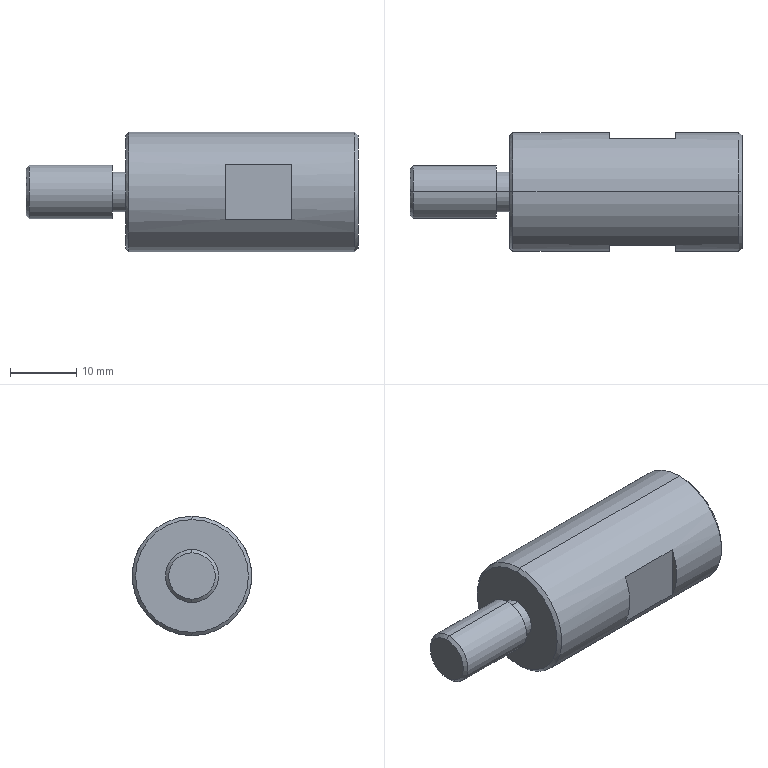Part | STEP file | PN_0032 Shaft_Default | 1 solid | 26 faces | box 50 x 18 x 18 mm | volume 8746 mm3 | plane 10 | cylinder 8 | cone 8 | commonest cylinder face diameters 6 x2 6.8 x2 8 x2 18 x2
STEP:
#1=CARTESIAN_POINT('',(0.,0.,0.));
#2=DIRECTION('',(0.,0.,1.));
#3=DIRECTION('',(1.,0.,0.));
#4=AXIS2_PLACEMENT_3D('',#1,#2,#3);
#5=CARTESIAN_POINT('',(-14.5,0.,-4.));
#6=VERTEX_POINT('',#5);
#7=CARTESIAN_POINT('',(-14.5,0.,4.));
#8=VERTEX_POINT('',#7);
#9=CARTESIAN_POINT('',(-14.5,0.,0.));
#10=DIRECTION('',(1.,0.,0.));
#11=DIRECTION('',(0.,0.,1.));
#12=AXIS2_PLACEMENT_3D('',#9,#10,#11);
#13=CIRCLE('',#12,4.);
#14=CARTESIAN_POINT('',(-15.,0.,0.));
#15=DIRECTION('',(1.,0.,0.));
#16=DIRECTION('',(0.,0.,-1.));
#17=AXIS2_PLACEMENT_3D('',#14,#15,#16);
#18=CYLINDRICAL_SURFACE('',#17,4.);
#19=CARTESIAN_POINT('',(-3.142,0.5));
#20=DIRECTION('',(1.,0.));
#21=VECTOR('',#20,1.);
#22=LINE('',#19,#21);
#23=(GEOMETRIC_REPRESENTATION_CONTEXT(2)PARAMETRIC_REPRESENTATION_CONTEXT()REPRESENTATION_CONTEXT('',''));
#24=DEFINITIONAL_REPRESENTATION('',(#22),#23);
#25=PCURVE('',#18,#24);
#26=CARTESIAN_POINT('',(-15.,0.,0.));
#27=DIRECTION('',(1.,0.,0.));
#28=DIRECTION('',(0.,0.,-1.));
#29=AXIS2_PLACEMENT_3D('',#26,#27,#28);
#30=CONICAL_SURFACE('',#29,3.5,0.7854);
#31=CARTESIAN_POINT('',(-3.142,0.5));
#32=DIRECTION('',(1.,0.));
#33=VECTOR('',#32,1.);
#34=LINE('',#31,#33);
#35=(GEOMETRIC_REPRESENTATION_CONTEXT(2)PARAMETRIC_REPRESENTATION_CONTEXT()REPRESENTATION_CONTEXT('',''));
#36=DEFINITIONAL_REPRESENTATION('',(#34),#35);
#37=PCURVE('',#30,#36);
#38=SURFACE_CURVE('',#13,(#25,#37),.PCURVE_S1.);
#39=EDGE_CURVE('',#6,#8,#38,.T.);
#40=ORIENTED_EDGE('',*,*,#39,.T.);
#41=CARTESIAN_POINT('',(-2.,0.,4.));
#42=VERTEX_POINT('',#41);
#43=CARTESIAN_POINT('',(-15.,0.,4.));
#44=DIRECTION('',(1.,0.,0.));
#45=VECTOR('',#44,1.);
#46=LINE('',#43,#45);
#47=CARTESIAN_POINT('',(3.142,0.));
#48=DIRECTION('',(0.,1.));
#49=VECTOR('',#48,1.);
#50=LINE('',#47,#49);
#51=(GEOMETRIC_REPRESENTATION_CONTEXT(2)PARAMETRIC_REPRESENTATION_CONTEXT()REPRESENTATION_CONTEXT('',''));
#52=DEFINITIONAL_REPRESENTATION('',(#50),#51);
#53=PCURVE('',#18,#52);
#54=CARTESIAN_POINT('',(-15.,0.,0.));
#55=DIRECTION('',(1.,0.,0.));
#56=DIRECTION('',(0.,0.,-1.));
#57=AXIS2_PLACEMENT_3D('',#54,#55,#56);
#58=CYLINDRICAL_SURFACE('',#57,4.);
#59=CARTESIAN_POINT('',(3.142,0.));
#60=DIRECTION('',(0.,1.));
#61=VECTOR('',#60,1.);
#62=LINE('',#59,#61);
#63=(GEOMETRIC_REPRESENTATION_CONTEXT(2)PARAMETRIC_REPRESENTATION_CONTEXT()REPRESENTATION_CONTEXT('',''));
#64=DEFINITIONAL_REPRESENTATION('',(#62),#63);
#65=PCURVE('',#58,#64);
#66=SURFACE_CURVE('',#46,(#53,#65),.PCURVE_S1.);
#67=EDGE_CURVE('',#8,#42,#66,.T.);
#68=ORIENTED_EDGE('',*,*,#67,.T.);
#69=CARTESIAN_POINT('',(-2.,0.,-4.));
#70=VERTEX_POINT('',#69);
#71=CARTESIAN_POINT('',(-2.,0.,0.));
#72=DIRECTION('',(-1.,0.,0.));
#73=DIRECTION('',(0.,0.,1.));
#74=AXIS2_PLACEMENT_3D('',#71,#72,#73);
#75=CIRCLE('',#74,4.);
#76=CARTESIAN_POINT('',(3.142,13.));
#77=DIRECTION('',(-1.,0.));
#78=VECTOR('',#77,1.);
#79=LINE('',#76,#78);
#80=(GEOMETRIC_REPRESENTATION_CONTEXT(2)PARAMETRIC_REPRESENTATION_CONTEXT()REPRESENTATION_CONTEXT('',''));
#81=DEFINITIONAL_REPRESENTATION('',(#79),#80);
#82=PCURVE('',#18,#81);
#83=CARTESIAN_POINT('',(-2.,0.,0.));
#84=DIRECTION('',(-1.,0.,0.));
#85=DIRECTION('',(0.,0.,1.));
#86=AXIS2_PLACEMENT_3D('',#83,#84,#85);
#87=PLANE('',#86);
#88=CARTESIAN_POINT('',(0.,0.));
#89=DIRECTION('',(1.,0.));
#90=AXIS2_PLACEMENT_2D('',#88,#89);
#91=CIRCLE('',#90,4.);
#92=(GEOMETRIC_REPRESENTATION_CONTEXT(2)PARAMETRIC_REPRESENTATION_CONTEXT()REPRESENTATION_CONTEXT('',''));
#93=DEFINITIONAL_REPRESENTATION('',(#91),#92);
#94=PCURVE('',#87,#93);
#95=SURFACE_CURVE('',#75,(#82,#94),.PCURVE_S1.);
#96=EDGE_CURVE('',#42,#70,#95,.T.);
#97=ORIENTED_EDGE('',*,*,#96,.T.);
#98=CARTESIAN_POINT('',(-15.,0.,-4.));
#99=DIRECTION('',(1.,0.,0.));
#100=VECTOR('',#99,1.);
#101=LINE('',#98,#100);
#102=CARTESIAN_POINT('',(0.,0.));
#103=DIRECTION('',(0.,1.));
#104=VECTOR('',#103,1.);
#105=LINE('',#102,#104);
#106=(GEOMETRIC_REPRESENTATION_CONTEXT(2)PARAMETRIC_REPRESENTATION_CONTEXT()REPRESENTATION_CONTEXT('',''));
#107=DEFINITIONAL_REPRESENTATION('',(#105),#106);
#108=PCURVE('',#18,#107);
#109=CARTESIAN_POINT('',(6.283,0.));
#110=DIRECTION('',(0.,1.));
#111=VECTOR('',#110,1.);
#112=LINE('',#109,#111);
#113=(GEOMETRIC_REPRESENTATION_CONTEXT(2)PARAMETRIC_REPRESENTATION_CONTEXT()REPRESENTATION_CONTEXT('',''));
#114=DEFINITIONAL_REPRESENTATION('',(#112),#113);
#115=PCURVE('',#58,#114);
#116=SURFACE_CURVE('',#101,(#108,#115),.PCURVE_S1.);
#117=EDGE_CURVE('',#6,#70,#116,.T.);
#118=ORIENTED_EDGE('',*,*,#117,.F.);
#119=EDGE_LOOP('',(#40,#68,#97,#118));
#120=FACE_BOUND('',#119,.T.);
#121=ADVANCED_FACE('',(#120),#18,.T.);
#122=CARTESIAN_POINT('',(-15.,0.,3.5));
#123=VERTEX_POINT('',#122);
#124=CARTESIAN_POINT('',(-15.,0.,-3.5));
#125=VERTEX_POINT('',#124);
#126=CARTESIAN_POINT('',(-15.,0.,0.));
#127=DIRECTION('',(-1.,0.,0.));
#128=DIRECTION('',(0.,0.,1.));
#129=AXIS2_PLACEMENT_3D('',#126,#127,#128);
#130=CIRCLE('',#129,3.5);
#131=CARTESIAN_POINT('',(3.142,0.));
#132=DIRECTION('',(-1.,0.));
#133=VECTOR('',#132,1.);
#134=LINE('',#131,#133);
#135=(GEOMETRIC_REPRESENTATION_CONTEXT(2)PARAMETRIC_REPRESENTATION_CONTEXT()REPRESENTATION_CONTEXT('',''));
#136=DEFINITIONAL_REPRESENTATION('',(#134),#135);
#137=PCURVE('',#30,#136);
#138=CARTESIAN_POINT('',(-15.,0.,0.));
#139=DIRECTION('',(-1.,0.,0.));
#140=DIRECTION('',(0.,0.,1.));
#141=AXIS2_PLACEMENT_3D('',#138,#139,#140);
#142=PLANE('',#141);
#143=CARTESIAN_POINT('',(0.,0.));
#144=DIRECTION('',(1.,0.));
#145=AXIS2_PLACEMENT_2D('',#143,#144);
#146=CIRCLE('',#145,3.5);
#147=(GEOMETRIC_REPRESENTATION_CONTEXT(2)PARAMETRIC_REPRESENTATION_CONTEXT()REPRESENTATION_CONTEXT('',''));
#148=DEFINITIONAL_REPRESENTATION('',(#146),#147);
#149=PCURVE('',#142,#148);
#150=SURFACE_CURVE('',#130,(#137,#149),.PCURVE_S1.);
#151=EDGE_CURVE('',#123,#125,#150,.T.);
#152=ORIENTED_EDGE('',*,*,#151,.F.);
#153=CARTESIAN_POINT('',(-15.,0.,3.5));
#154=DIRECTION('',(0.7071,0.,0.7071));
#155=VECTOR('',#154,1.);
#156=LINE('',#153,#155);
#157=CARTESIAN_POINT('',(3.142,0.));
#158=DIRECTION('',(0.,1.));
#159=VECTOR('',#158,1.);
#160=LINE('',#157,#159);
#161=(GEOMETRIC_REPRESENTATION_CONTEXT(2)PARAMETRIC_REPRESENTATION_CONTEXT()REPRESENTATION_CONTEXT('',''));
#162=DEFINITIONAL_REPRESENTATION('',(#160),#161);
#163=PCURVE('',#30,#162);
#164=CARTESIAN_POINT('',(-15.,0.,0.));
#165=DIRECTION('',(1.,0.,0.));
#166=DIRECTION('',(0.,0.,-1.));
#167=AXIS2_PLACEMENT_3D('',#164,#165,#166);
#168=CONICAL_SURFACE('',#167,3.5,0.7854);
#169=CARTESIAN_POINT('',(3.142,0.));
#170=DIRECTION('',(0.,1.));
#171=VECTOR('',#170,1.);
#172=LINE('',#169,#171);
#173=(GEOMETRIC_REPRESENTATION_CONTEXT(2)PARAMETRIC_REPRESENTATION_CONTEXT()REPRESENTATION_CONTEXT('',''));
#174=DEFINITIONAL_REPRESENTATION('',(#172),#173);
#175=PCURVE('',#168,#174);
#176=SURFACE_CURVE('',#156,(#163,#175),.PCURVE_S1.);
#177=EDGE_CURVE('',#123,#8,#176,.T.);
#178=ORIENTED_EDGE('',*,*,#177,.T.);
#179=ORIENTED_EDGE('',*,*,#39,.F.);
#180=CARTESIAN_POINT('',(-15.,0.,-3.5));
#181=DIRECTION('',(0.7071,0.,-0.7071));
#182=VECTOR('',#181,1.);
#183=LINE('',#180,#182);
#184=CARTESIAN_POINT('',(0.,0.));
#185=DIRECTION('',(0.,1.));
#186=VECTOR('',#185,1.);
#187=LINE('',#184,#186);
#188=(GEOMETRIC_REPRESENTATION_CONTEXT(2)PARAMETRIC_REPRESENTATION_CONTEXT()REPRESENTATION_CONTEXT('',''));
#189=DEFINITIONAL_REPRESENTATION('',(#187),#188);
#190=PCURVE('',#30,#189);
#191=CARTESIAN_POINT('',(6.283,0.));
#192=DIRECTION('',(0.,1.));
#193=VECTOR('',#192,1.);
#194=LINE('',#191,#193);
#195=(GEOMETRIC_REPRESENTATION_CONTEXT(2)PARAMETRIC_REPRESENTATION_CONTEXT()REPRESENTATION_CONTEXT('',''));
#196=DEFINITIONAL_REPRESENTATION('',(#194),#195);
#197=PCURVE('',#168,#196);
#198=SURFACE_CURVE('',#183,(#190,#197),.PCURVE_S1.);
#199=EDGE_CURVE('',#125,#6,#198,.T.);
#200=ORIENTED_EDGE('',*,*,#199,.F.);
#201=EDGE_LOOP('',(#152,#178,#179,#200));
#202=FACE_BOUND('',#201,.T.);
#203=ADVANCED_FACE('',(#202),#30,.T.);
#204=CARTESIAN_POINT('',(-2.,0.,3.));
#205=VERTEX_POINT('',#204);
#206=CARTESIAN_POINT('',(-2.,0.,-3.));
#207=VERTEX_POINT('',#206);
#208=CARTESIAN_POINT('',(-2.,0.,0.));
#209=DIRECTION('',(-1.,0.,0.));
#210=DIRECTION('',(0.,0.,1.));
#211=AXIS2_PLACEMENT_3D('',#208,#209,#210);
#212=CIRCLE('',#211,3.);
#213=CARTESIAN_POINT('',(-2.,0.,0.));
#214=DIRECTION('',(1.,0.,0.));
#215=DIRECTION('',(0.,0.,-1.));
#216=AXIS2_PLACEMENT_3D('',#213,#214,#215);
#217=CYLINDRICAL_SURFACE('',#216,3.);
#218=CARTESIAN_POINT('',(3.142,0.));
#219=DIRECTION('',(-1.,0.));
#220=VECTOR('',#219,1.);
#221=LINE('',#218,#220);
#222=(GEOMETRIC_REPRESENTATION_CONTEXT(2)PARAMETRIC_REPRESENTATION_CONTEXT()REPRESENTATION_CONTEXT('',''));
#223=DEFINITIONAL_REPRESENTATION('',(#221),#222);
#224=PCURVE('',#217,#223);
#225=CARTESIAN_POINT('',(0.,0.));
#226=DIRECTION('',(1.,0.));
#227=AXIS2_PLACEMENT_2D('',#225,#226);
#228=CIRCLE('',#227,3.);
#229=(GEOMETRIC_REPRESENTATION_CONTEXT(2)PARAMETRIC_REPRESENTATION_CONTEXT()REPRESENTATION_CONTEXT('',''));
#230=DEFINITIONAL_REPRESENTATION('',(#228),#229);
#231=PCURVE('',#87,#230);
#232=SURFACE_CURVE('',#212,(#224,#231),.PCURVE_S1.);
#233=EDGE_CURVE('',#205,#207,#232,.T.);
#234=ORIENTED_EDGE('',*,*,#233,.F.);
#235=CARTESIAN_POINT('',(0.,0.,3.));
#236=VERTEX_POINT('',#235);
#237=CARTESIAN_POINT('',(-2.,0.,3.));
#238=DIRECTION('',(1.,0.,0.));
#239=VECTOR('',#238,1.);
#240=LINE('',#237,#239);
#241=CARTESIAN_POINT('',(3.142,0.));
#242=DIRECTION('',(0.,1.));
#243=VECTOR('',#242,1.);
#244=LINE('',#241,#243);
#245=(GEOMETRIC_REPRESENTATION_CONTEXT(2)PARAMETRIC_REPRESENTATION_CONTEXT()REPRESENTATION_CONTEXT('',''));
#246=DEFINITIONAL_REPRESENTATION('',(#244),#245);
#247=PCURVE('',#217,#246);
#248=CARTESIAN_POINT('',(-2.,0.,0.));
#249=DIRECTION('',(1.,0.,0.));
#250=DIRECTION('',(0.,0.,-1.));
#251=AXIS2_PLACEMENT_3D('',#248,#249,#250);
#252=CYLINDRICAL_SURFACE('',#251,3.);
#253=CARTESIAN_POINT('',(3.142,0.));
#254=DIRECTION('',(0.,1.));
#255=VECTOR('',#254,1.);
#256=LINE('',#253,#255);
#257=(GEOMETRIC_REPRESENTATION_CONTEXT(2)PARAMETRIC_REPRESENTATION_CONTEXT()REPRESENTATION_CONTEXT('',''));
#258=DEFINITIONAL_REPRESENTATION('',(#256),#257);
#259=PCURVE('',#252,#258);
#260=SURFACE_CURVE('',#240,(#247,#259),.PCURVE_S1.);
#261=EDGE_CURVE('',#205,#236,#260,.T.);
#262=ORIENTED_EDGE('',*,*,#261,.T.);
#263=CARTESIAN_POINT('',(0.,0.,-3.));
#264=VERTEX_POINT('',#263);
#265=CARTESIAN_POINT('',(0.,0.,0.));
#266=DIRECTION('',(-1.,0.,0.));
#267=DIRECTION('',(0.,0.,1.));
#268=AXIS2_PLACEMENT_3D('',#265,#266,#267);
#269=CIRCLE('',#268,3.);
#270=CARTESIAN_POINT('',(3.142,2.));
#271=DIRECTION('',(-1.,0.));
#272=VECTOR('',#271,1.);
#273=LINE('',#270,#272);
#274=(GEOMETRIC_REPRESENTATION_CONTEXT(2)PARAMETRIC_REPRESENTATION_CONTEXT()REPRESENTATION_CONTEXT('',''));
#275=DEFINITIONAL_REPRESENTATION('',(#273),#274);
#276=PCURVE('',#217,#275);
#277=CARTESIAN_POINT('',(0.,0.,0.));
#278=DIRECTION('',(1.,0.,0.));
#279=DIRECTION('',(0.,0.,-1.));
#280=AXIS2_PLACEMENT_3D('',#277,#278,#279);
#281=PLANE('',#280);
#282=CARTESIAN_POINT('',(-3.,0.));
#283=CARTESIAN_POINT('',(-3.,5.196));
#284=CARTESIAN_POINT('',(1.5,2.598));
#285=CARTESIAN_POINT('',(6.,0.));
#286=CARTESIAN_POINT('',(1.5,-2.598));
#287=CARTESIAN_POINT('',(-3.,-5.196));
#288=CARTESIAN_POINT('',(-3.,0.));
#289=(BOUNDED_CURVE()B_SPLINE_CURVE(2,(#282,#283,#284,#285,#286,#287,#288),.UNSPECIFIED.,.T.,.F.)B_SPLINE_CURVE_WITH_KNOTS((1,2,2,2,2,1),(-2.094,0.,2.094,4.189,6.283,8.378),.UNSPECIFIED.)CURVE()GEOMETRIC_REPRESENTATION_ITEM()RATIONAL_B_SPLINE_CURVE((1.,0.5,1.,0.5,1.,0.5,1.))REPRESENTATION_ITEM(''));
#290=(GEOMETRIC_REPRESENTATION_CONTEXT(2)PARAMETRIC_REPRESENTATION_CONTEXT()REPRESENTATION_CONTEXT('',''));
#291=DEFINITIONAL_REPRESENTATION('',(#289),#290);
#292=PCURVE('',#281,#291);
#293=SURFACE_CURVE('',#269,(#276,#292),.PCURVE_S1.);
#294=EDGE_CURVE('',#236,#264,#293,.T.);
#295=ORIENTED_EDGE('',*,*,#294,.T.);
#296=CARTESIAN_POINT('',(-2.,0.,-3.));
#297=DIRECTION('',(1.,0.,0.));
#298=VECTOR('',#297,1.);
#299=LINE('',#296,#298);
#300=CARTESIAN_POINT('',(0.,0.));
#301=DIRECTION('',(0.,1.));
#302=VECTOR('',#301,1.);
#303=LINE('',#300,#302);
#304=(GEOMETRIC_REPRESENTATION_CONTEXT(2)PARAMETRIC_REPRESENTATION_CONTEXT()REPRESENTATION_CONTEXT('',''));
#305=DEFINITIONAL_REPRESENTATION('',(#303),#304);
#306=PCURVE('',#217,#305);
#307=CARTESIAN_POINT('',(6.283,0.));
#308=DIRECTION('',(0.,1.));
#309=VECTOR('',#308,1.);
#310=LINE('',#307,#309);
#311=(GEOMETRIC_REPRESENTATION_CONTEXT(2)PARAMETRIC_REPRESENTATION_CONTEXT()REPRESENTATION_CONTEXT('',''));
#312=DEFINITIONAL_REPRESENTATION('',(#310),#311);
#313=PCURVE('',#252,#312);
#314=SURFACE_CURVE('',#299,(#306,#313),.PCURVE_S1.);
#315=EDGE_CURVE('',#207,#264,#314,.T.);
#316=ORIENTED_EDGE('',*,*,#315,.F.);
#317=EDGE_LOOP('',(#234,#262,#295,#316));
#318=FACE_BOUND('',#317,.T.);
#319=ADVANCED_FACE('',(#318),#217,.T.);
#320=CARTESIAN_POINT('',(35.,0.,-8.5));
#321=VERTEX_POINT('',#320);
#322=CARTESIAN_POINT('',(35.,0.,8.5));
#323=VERTEX_POINT('',#322);
#324=CARTESIAN_POINT('',(35.,0.,0.));
#325=DIRECTION('',(1.,0.,0.));
#326=DIRECTION('',(0.,0.,-1.));
#327=AXIS2_PLACEMENT_3D('',#324,#325,#326);
#328=CIRCLE('',#327,8.5);
#329=CARTESIAN_POINT('',(35.,0.,0.));
#330=DIRECTION('',(-1.,0.,0.));
#331=DIRECTION('',(0.,0.,1.));
#332=AXIS2_PLACEMENT_3D('',#329,#330,#331);
#333=CONICAL_SURFACE('',#332,8.5,0.7854);
#334=CARTESIAN_POINT('',(3.142,0.));
#335=DIRECTION('',(-1.,0.));
#336=VECTOR('',#335,1.);
#337=LINE('',#334,#336);
#338=(GEOMETRIC_REPRESENTATION_CONTEXT(2)PARAMETRIC_REPRESENTATION_CONTEXT()REPRESENTATION_CONTEXT('',''));
#339=DEFINITIONAL_REPRESENTATION('',(#337),#338);
#340=PCURVE('',#333,#339);
#341=CARTESIAN_POINT('',(35.,0.,0.));
#342=DIRECTION('',(1.,0.,0.));
#343=DIRECTION('',(0.,0.,-1.));
#344=AXIS2_PLACEMENT_3D('',#341,#342,#343);
#345=PLANE('',#344);
#346=CARTESIAN_POINT('',(0.,0.));
#347=DIRECTION('',(1.,0.));
#348=AXIS2_PLACEMENT_2D('',#346,#347);
#349=CIRCLE('',#348,8.5);
#350=(GEOMETRIC_REPRESENTATION_CONTEXT(2)PARAMETRIC_REPRESENTATION_CONTEXT()REPRESENTATION_CONTEXT('',''));
#351=DEFINITIONAL_REPRESENTATION('',(#349),#350);
#352=PCURVE('',#345,#351);
#353=SURFACE_CURVE('',#328,(#340,#352),.PCURVE_S1.);
#354=EDGE_CURVE('',#321,#323,#353,.T.);
#355=ORIENTED_EDGE('',*,*,#354,.F.);
#356=CARTESIAN_POINT('',(34.5,0.,-9.));
#357=VERTEX_POINT('',#356);
#358=CARTESIAN_POINT('',(35.,0.,-8.5));
#359=DIRECTION('',(-0.7071,0.,-0.7071));
#360=VECTOR('',#359,1.);
#361=LINE('',#358,#360);
#362=CARTESIAN_POINT('',(3.142,0.));
#363=DIRECTION('',(0.,1.));
#364=VECTOR('',#363,1.);
#365=LINE('',#362,#364);
#366=(GEOMETRIC_REPRESENTATION_CONTEXT(2)PARAMETRIC_REPRESENTATION_CONTEXT()REPRESENTATION_CONTEXT('',''));
#367=DEFINITIONAL_REPRESENTATION('',(#365),#366);
#368=PCURVE('',#333,#367);
#369=CARTESIAN_POINT('',(35.,0.,0.));
#370=DIRECTION('',(-1.,0.,0.));
#371=DIRECTION('',(0.,0.,1.));
#372=AXIS2_PLACEMENT_3D('',#369,#370,#371);
#373=CONICAL_SURFACE('',#372,8.5,0.7854);
#374=CARTESIAN_POINT('',(3.142,0.));
#375=DIRECTION('',(0.,1.));
#376=VECTOR('',#375,1.);
#377=LINE('',#374,#376);
#378=(GEOMETRIC_REPRESENTATION_CONTEXT(2)PARAMETRIC_REPRESENTATION_CONTEXT()REPRESENTATION_CONTEXT('',''));
#379=DEFINITIONAL_REPRESENTATION('',(#377),#378);
#380=PCURVE('',#373,#379);
#381=SURFACE_CURVE('',#361,(#368,#380),.PCURVE_S1.);
#382=EDGE_CURVE('',#321,#357,#381,.T.);
#383=ORIENTED_EDGE('',*,*,#382,.T.);
#384=CARTESIAN_POINT('',(34.5,0.,9.));
#385=VERTEX_POINT('',#384);
#386=CARTESIAN_POINT('',(34.5,0.,0.));
#387=DIRECTION('',(-1.,0.,0.));
#388=DIRECTION('',(0.,0.,-1.));
#389=AXIS2_PLACEMENT_3D('',#386,#387,#388);
#390=CIRCLE('',#389,9.);
#391=CARTESIAN_POINT('',(-3.142,0.5));
#392=DIRECTION('',(1.,0.));
#393=VECTOR('',#392,1.);
#394=LINE('',#391,#393);
#395=(GEOMETRIC_REPRESENTATION_CONTEXT(2)PARAMETRIC_REPRESENTATION_CONTEXT()REPRESENTATION_CONTEXT('',''));
#396=DEFINITIONAL_REPRESENTATION('',(#394),#395);
#397=PCURVE('',#333,#396);
#398=CARTESIAN_POINT('',(35.,0.,0.));
#399=DIRECTION('',(-1.,0.,0.));
#400=DIRECTION('',(0.,0.,1.));
#401=AXIS2_PLACEMENT_3D('',#398,#399,#400);
#402=CYLINDRICAL_SURFACE('',#401,9.);
#403=CARTESIAN_POINT('',(-3.142,0.5));
#404=DIRECTION('',(1.,0.));
#405=VECTOR('',#404,1.);
#406=LINE('',#403,#405);
#407=(GEOMETRIC_REPRESENTATION_CONTEXT(2)PARAMETRIC_REPRESENTATION_CONTEXT()REPRESENTATION_CONTEXT('',''));
#408=DEFINITIONAL_REPRESENTATION('',(#406),#407);
#409=PCURVE('',#402,#408);
#410=SURFACE_CURVE('',#390,(#397,#409),.PCURVE_S1.);
#411=EDGE_CURVE('',#385,#357,#410,.T.);
#412=ORIENTED_EDGE('',*,*,#411,.F.);
#413=CARTESIAN_POINT('',(35.,0.,8.5));
#414=DIRECTION('',(-0.7071,0.,0.7071));
#415=VECTOR('',#414,1.);
#416=LINE('',#413,#415);
#417=CARTESIAN_POINT('',(0.,0.));
#418=DIRECTION('',(0.,1.));
#419=VECTOR('',#418,1.);
#420=LINE('',#417,#419);
#421=(GEOMETRIC_REPRESENTATION_CONTEXT(2)PARAMETRIC_REPRESENTATION_CONTEXT()REPRESENTATION_CONTEXT('',''));
#422=DEFINITIONAL_REPRESENTATION('',(#420),#421);
#423=PCURVE('',#333,#422);
#424=CARTESIAN_POINT('',(6.283,0.));
#425=DIRECTION('',(0.,1.));
#426=VECTOR('',#425,1.);
#427=LINE('',#424,#426);
#428=(GEOMETRIC_REPRESENTATION_CONTEXT(2)PARAMETRIC_REPRESENTATION_CONTEXT()REPRESENTATION_CONTEXT('',''));
#429=DEFINITIONAL_REPRESENTATION('',(#427),#428);
#430=PCURVE('',#373,#429);
#431=SURFACE_CURVE('',#416,(#423,#430),.PCURVE_S1.);
#432=EDGE_CURVE('',#323,#385,#431,.T.);
#433=ORIENTED_EDGE('',*,*,#432,.F.);
#434=EDGE_LOOP('',(#355,#383,#412,#433));
#435=FACE_BOUND('',#434,.T.);
#436=ADVANCED_FACE('',(#435),#333,.T.);
#437=CARTESIAN_POINT('',(0.,0.,8.5));
#438=VERTEX_POINT('',#437);
#439=CARTESIAN_POINT('',(0.,0.,-8.5));
#440=VERTEX_POINT('',#439);
#441=CARTESIAN_POINT('',(0.,0.,0.));
#442=DIRECTION('',(-1.,0.,0.));
#443=DIRECTION('',(0.,0.,-1.));
#444=AXIS2_PLACEMENT_3D('',#441,#442,#443);
#445=CIRCLE('',#444,8.5);
#446=CARTESIAN_POINT('',(0.5,0.,0.));
#447=DIRECTION('',(1.,0.,0.));
#448=DIRECTION('',(0.,0.,-1.));
#449=AXIS2_PLACEMENT_3D('',#446,#447,#448);
#450=CONICAL_SURFACE('',#449,9.,0.7854);
#451=CARTESIAN_POINT('',(6.283,-0.5));
#452=DIRECTION('',(-1.,0.));
#453=VECTOR('',#452,1.);
#454=LINE('',#451,#453);
#455=(GEOMETRIC_REPRESENTATION_CONTEXT(2)PARAMETRIC_REPRESENTATION_CONTEXT()REPRESENTATION_CONTEXT('',''));
#456=DEFINITIONAL_REPRESENTATION('',(#454),#455);
#457=PCURVE('',#450,#456);
#458=CARTESIAN_POINT('',(8.5,0.));
#459=CARTESIAN_POINT('',(8.5,-14.722));
#460=CARTESIAN_POINT('',(-4.25,-7.361));
#461=CARTESIAN_POINT('',(-17.,0.));
#462=CARTESIAN_POINT('',(-4.25,7.361));
#463=CARTESIAN_POINT('',(8.5,14.722));
#464=CARTESIAN_POINT('',(8.5,0.));
#465=(BOUNDED_CURVE()B_SPLINE_CURVE(2,(#458,#459,#460,#461,#462,#463,#464),.UNSPECIFIED.,.T.,.F.)B_SPLINE_CURVE_WITH_KNOTS((1,2,2,2,2,1),(-2.094,0.,2.094,4.189,6.283,8.378),.UNSPECIFIED.)CURVE()GEOMETRIC_REPRESENTATION_ITEM()RATIONAL_B_SPLINE_CURVE((1.,0.5,1.,0.5,1.,0.5,1.))REPRESENTATION_ITEM(''));
#466=(GEOMETRIC_REPRESENTATION_CONTEXT(2)PARAMETRIC_REPRESENTATION_CONTEXT()REPRESENTATION_CONTEXT('',''));
#467=DEFINITIONAL_REPRESENTATION('',(#465),#466);
#468=PCURVE('',#281,#467);
#469=SURFACE_CURVE('',#445,(#457,#468),.PCURVE_S1.);
#470=EDGE_CURVE('',#438,#440,#469,.T.);
#471=ORIENTED_EDGE('',*,*,#470,.F.);
#472=CARTESIAN_POINT('',(0.5,0.,9.));
#473=VERTEX_POINT('',#472);
#474=CARTESIAN_POINT('',(0.5,0.,9.));
#475=DIRECTION('',(0.7071,0.,0.7071));
#476=VECTOR('',#475,1.);
#477=LINE('',#474,#476);
#478=CARTESIAN_POINT('',(3.142,0.));
#479=DIRECTION('',(0.,1.));
#480=VECTOR('',#479,1.);
#481=LINE('',#478,#480);
#482=(GEOMETRIC_REPRESENTATION_CONTEXT(2)PARAMETRIC_REPRESENTATION_CONTEXT()REPRESENTATION_CONTEXT('',''));
#483=DEFINITIONAL_REPRESENTATION('',(#481),#482);
#484=PCURVE('',#450,#483);
#485=CARTESIAN_POINT('',(0.5,0.,0.));
#486=DIRECTION('',(1.,0.,0.));
#487=DIRECTION('',(0.,0.,-1.));
#488=AXIS2_PLACEMENT_3D('',#485,#486,#487);
#489=CONICAL_SURFACE('',#488,9.,0.7854);
#490=CARTESIAN_POINT('',(3.142,0.));
#491=DIRECTION('',(0.,1.));
#492=VECTOR('',#491,1.);
#493=LINE('',#490,#492);
#494=(GEOMETRIC_REPRESENTATION_CONTEXT(2)PARAMETRIC_REPRESENTATION_CONTEXT()REPRESENTATION_CONTEXT('',''));
#495=DEFINITIONAL_REPRESENTATION('',(#493),#494);
#496=PCURVE('',#489,#495);
#497=SURFACE_CURVE('',#477,(#484,#496),.PCURVE_S1.);
#498=EDGE_CURVE('',#438,#473,#497,.T.);
#499=ORIENTED_EDGE('',*,*,#498,.T.);
#500=CARTESIAN_POINT('',(0.5,0.,-9.));
#501=VERTEX_POINT('',#500);
#502=CARTESIAN_POINT('',(0.5,0.,0.));
#503=DIRECTION('',(1.,0.,0.));
#504=DIRECTION('',(0.,0.,-1.));
#505=AXIS2_PLACEMENT_3D('',#502,#503,#504);
#506=CIRCLE('',#505,9.);
#507=CARTESIAN_POINT('',(0.,0.));
#508=DIRECTION('',(1.,0.));
#509=VECTOR('',#508,1.);
#510=LINE('',#507,#509);
#511=(GEOMETRIC_REPRESENTATION_CONTEXT(2)PARAMETRIC_REPRESENTATION_CONTEXT()REPRESENTATION_CONTEXT('',''));
#512=DEFINITIONAL_REPRESENTATION('',(#510),#511);
#513=PCURVE('',#450,#512);
#514=CARTESIAN_POINT('',(3.142,34.5));
#515=DIRECTION('',(-1.,0.));
#516=VECTOR('',#515,1.);
#517=LINE('',#514,#516);
#518=(GEOMETRIC_REPRESENTATION_CONTEXT(2)PARAMETRIC_REPRESENTATION_CONTEXT()REPRESENTATION_CONTEXT('',''));
#519=DEFINITIONAL_REPRESENTATION('',(#517),#518);
#520=PCURVE('',#402,#519);
#521=SURFACE_CURVE('',#506,(#513,#520),.PCURVE_S1.);
#522=EDGE_CURVE('',#501,#473,#521,.T.);
#523=ORIENTED_EDGE('',*,*,#522,.F.);
#524=CARTESIAN_POINT('',(0.5,0.,-9.));
#525=DIRECTION('',(0.7071,0.,-0.7071));
#526=VECTOR('',#525,1.);
#527=LINE('',#524,#526);
#528=CARTESIAN_POINT('',(0.,0.));
#529=DIRECTION('',(0.,1.));
#530=VECTOR('',#529,1.);
#531=LINE('',#528,#530);
#532=(GEOMETRIC_REPRESENTATION_CONTEXT(2)PARAMETRIC_REPRESENTATION_CONTEXT()REPRESENTATION_CONTEXT('',''));
#533=DEFINITIONAL_REPRESENTATION('',(#531),#532);
#534=PCURVE('',#450,#533);
#535=CARTESIAN_POINT('',(6.283,0.));
#536=DIRECTION('',(0.,1.));
#537=VECTOR('',#536,1.);
#538=LINE('',#535,#537);
#539=(GEOMETRIC_REPRESENTATION_CONTEXT(2)PARAMETRIC_REPRESENTATION_CONTEXT()REPRESENTATION_CONTEXT('',''));
#540=DEFINITIONAL_REPRESENTATION('',(#538),#539);
#541=PCURVE('',#489,#540);
#542=SURFACE_CURVE('',#527,(#534,#541),.PCURVE_S1.);
#543=EDGE_CURVE('',#440,#501,#542,.T.);
#544=ORIENTED_EDGE('',*,*,#543,.F.);
#545=EDGE_LOOP('',(#471,#499,#523,#544));
#546=FACE_BOUND('',#545,.T.);
#547=ADVANCED_FACE('',(#546),#450,.T.);
#548=CARTESIAN_POINT('',(15.25,0.,-3.4));
#549=VERTEX_POINT('',#548);
#550=CARTESIAN_POINT('',(35.,0.,-3.4));
#551=VERTEX_POINT('',#550);
#552=CARTESIAN_POINT('',(35.,0.,-3.4));
#553=DIRECTION('',(1.,0.,0.));
#554=VECTOR('',#553,1.);
#555=LINE('',#552,#554);
#556=CARTESIAN_POINT('',(35.,0.,0.));
#557=DIRECTION('',(1.,0.,0.));
#558=DIRECTION('',(0.,0.,-1.));
#559=AXIS2_PLACEMENT_3D('',#556,#557,#558);
#560=CYLINDRICAL_SURFACE('',#559,3.4);
#561=CARTESIAN_POINT('',(6.283,0.));
#562=DIRECTION('',(0.,1.));
#563=VECTOR('',#562,1.);
#564=LINE('',#561,#563);
#565=(GEOMETRIC_REPRESENTATION_CONTEXT(2)PARAMETRIC_REPRESENTATION_CONTEXT()REPRESENTATION_CONTEXT('',''));
#566=DEFINITIONAL_REPRESENTATION('',(#564),#565);
#567=PCURVE('',#560,#566);
#568=CARTESIAN_POINT('',(35.,0.,0.));
#569=DIRECTION('',(1.,0.,0.));
#570=DIRECTION('',(0.,0.,-1.));
#571=AXIS2_PLACEMENT_3D('',#568,#569,#570);
#572=CYLINDRICAL_SURFACE('',#571,3.4);
#573=CARTESIAN_POINT('',(0.,0.));
#574=DIRECTION('',(0.,1.));
#575=VECTOR('',#574,1.);
#576=LINE('',#573,#575);
#577=(GEOMETRIC_REPRESENTATION_CONTEXT(2)PARAMETRIC_REPRESENTATION_CONTEXT()REPRESENTATION_CONTEXT('',''));
#578=DEFINITIONAL_REPRESENTATION('',(#576),#577);
#579=PCURVE('',#572,#578);
#580=SURFACE_CURVE('',#555,(#567,#579),.PCURVE_S1.);
#581=EDGE_CURVE('',#549,#551,#580,.T.);
#582=ORIENTED_EDGE('',*,*,#581,.T.);
#583=CARTESIAN_POINT('',(35.,0.,3.4));
#584=VERTEX_POINT('',#583);
#585=CARTESIAN_POINT('',(35.,0.,0.));
#586=DIRECTION('',(1.,0.,0.));
#587=DIRECTION('',(0.,0.,-1.));
#588=AXIS2_PLACEMENT_3D('',#585,#586,#587);
#589=CIRCLE('',#588,3.4);
#590=CARTESIAN_POINT('',(0.,0.));
#591=DIRECTION('',(1.,0.));
#592=VECTOR('',#591,1.);
#593=LINE('',#590,#592);
#594=(GEOMETRIC_REPRESENTATION_CONTEXT(2)PARAMETRIC_REPRESENTATION_CONTEXT()REPRESENTATION_CONTEXT('',''));
#595=DEFINITIONAL_REPRESENTATION('',(#593),#594);
#596=PCURVE('',#560,#595);
#597=CARTESIAN_POINT('',(0.,0.));
#598=DIRECTION('',(1.,0.));
#599=AXIS2_PLACEMENT_2D('',#597,#598);
#600=CIRCLE('',#599,3.4);
#601=(GEOMETRIC_REPRESENTATION_CONTEXT(2)PARAMETRIC_REPRESENTATION_CONTEXT()REPRESENTATION_CONTEXT('',''));
#602=DEFINITIONAL_REPRESENTATION('',(#600),#601);
#603=PCURVE('',#345,#602);
#604=SURFACE_CURVE('',#589,(#596,#603),.PCURVE_S1.);
#605=EDGE_CURVE('',#584,#551,#604,.T.);
#606=ORIENTED_EDGE('',*,*,#605,.F.);
#607=CARTESIAN_POINT('',(15.25,0.,3.4));
#608=VERTEX_POINT('',#607);
#609=CARTESIAN_POINT('',(35.,0.,3.4));
#610=DIRECTION('',(1.,0.,0.));
#611=VECTOR('',#610,1.);
#612=LINE('',#609,#611);
#613=CARTESIAN_POINT('',(3.142,0.));
#614=DIRECTION('',(0.,1.));
#615=VECTOR('',#614,1.);
#616=LINE('',#613,#615);
#617=(GEOMETRIC_REPRESENTATION_CONTEXT(2)PARAMETRIC_REPRESENTATION_CONTEXT()REPRESENTATION_CONTEXT('',''));
#618=DEFINITIONAL_REPRESENTATION('',(#616),#617);
#619=PCURVE('',#560,#618);
#620=CARTESIAN_POINT('',(3.142,0.));
#621=DIRECTION('',(0.,1.));
#622=VECTOR('',#621,1.);
#623=LINE('',#620,#622);
#624=(GEOMETRIC_REPRESENTATION_CONTEXT(2)PARAMETRIC_REPRESENTATION_CONTEXT()REPRESENTATION_CONTEXT('',''));
#625=DEFINITIONAL_REPRESENTATION('',(#623),#624);
#626=PCURVE('',#572,#625);
#627=SURFACE_CURVE('',#612,(#619,#626),.PCURVE_S1.);
#628=EDGE_CURVE('',#608,#584,#627,.T.);
#629=ORIENTED_EDGE('',*,*,#628,.F.);
#630=CARTESIAN_POINT('',(15.25,0.,0.));
#631=DIRECTION('',(1.,0.,0.));
#632=DIRECTION('',(0.,0.,-1.));
#633=AXIS2_PLACEMENT_3D('',#630,#631,#632);
#634=CIRCLE('',#633,3.4);
#635=CARTESIAN_POINT('',(0.,-19.75));
#636=DIRECTION('',(1.,0.));
#637=VECTOR('',#636,1.);
#638=LINE('',#635,#637);
#639=(GEOMETRIC_REPRESENTATION_CONTEXT(2)PARAMETRIC_REPRESENTATION_CONTEXT()REPRESENTATION_CONTEXT('',''));
#640=DEFINITIONAL_REPRESENTATION('',(#638),#639);
#641=PCURVE('',#560,#640);
#642=CARTESIAN_POINT('',(15.25,0.,0.));
#643=DIRECTION('',(1.,0.,0.));
#644=DIRECTION('',(0.,0.,-1.));
#645=AXIS2_PLACEMENT_3D('',#642,#643,#644);
#646=CONICAL_SURFACE('',#645,3.4,1.03);
#647=CARTESIAN_POINT('',(0.,0.));
#648=DIRECTION('',(1.,0.));
#649=VECTOR('',#648,1.);
#650=LINE('',#647,#649);
#651=(GEOMETRIC_REPRESENTATION_CONTEXT(2)PARAMETRIC_REPRESENTATION_CONTEXT()REPRESENTATION_CONTEXT('',''));
#652=DEFINITIONAL_REPRESENTATION('',(#650),#651);
#653=PCURVE('',#646,#652);
#654=SURFACE_CURVE('',#634,(#641,#653),.PCURVE_S1.);
#655=EDGE_CURVE('',#608,#549,#654,.T.);
#656=ORIENTED_EDGE('',*,*,#655,.T.);
#657=EDGE_LOOP('',(#582,#606,#629,#656));
#658=FACE_BOUND('',#657,.F.);
#659=ADVANCED_FACE('',(#658),#560,.F.);
#660=ORIENTED_EDGE('',*,*,#655,.F.);
#661=CARTESIAN_POINT('',(13.207,0.,0.));
#662=VERTEX_POINT('',#661);
#663=CARTESIAN_POINT('',(15.25,0.,3.4));
#664=DIRECTION('',(0.515,0.,0.8572));
#665=VECTOR('',#664,1.);
#666=LINE('',#663,#665);
#667=CARTESIAN_POINT('',(3.142,0.));
#668=DIRECTION('',(0.,1.));
#669=VECTOR('',#668,1.);
#670=LINE('',#667,#669);
#671=(GEOMETRIC_REPRESENTATION_CONTEXT(2)PARAMETRIC_REPRESENTATION_CONTEXT()REPRESENTATION_CONTEXT('',''));
#672=DEFINITIONAL_REPRESENTATION('',(#670),#671);
#673=PCURVE('',#646,#672);
#674=CARTESIAN_POINT('',(15.25,0.,0.));
#675=DIRECTION('',(1.,0.,0.));
#676=DIRECTION('',(0.,0.,-1.));
#677=AXIS2_PLACEMENT_3D('',#674,#675,#676);
#678=CONICAL_SURFACE('',#677,3.4,1.03);
#679=CARTESIAN_POINT('',(3.142,0.));
#680=DIRECTION('',(0.,1.));
#681=VECTOR('',#680,1.);
#682=LINE('',#679,#681);
#683=(GEOMETRIC_REPRESENTATION_CONTEXT(2)PARAMETRIC_REPRESENTATION_CONTEXT()REPRESENTATION_CONTEXT('',''));
#684=DEFINITIONAL_REPRESENTATION('',(#682),#683);
#685=PCURVE('',#678,#684);
#686=SURFACE_CURVE('',#666,(#673,#685),.PCURVE_S1.);
#687=EDGE_CURVE('',#662,#608,#686,.T.);
#688=ORIENTED_EDGE('',*,*,#687,.F.);
#689=CARTESIAN_POINT('',(15.25,0.,-3.4));
#690=DIRECTION('',(0.515,0.,-0.8572));
#691=VECTOR('',#690,1.);
#692=LINE('',#689,#691);
#693=CARTESIAN_POINT('',(6.283,0.));
#694=DIRECTION('',(0.,1.));
#695=VECTOR('',#694,1.);
#696=LINE('',#693,#695);
#697=(GEOMETRIC_REPRESENTATION_CONTEXT(2)PARAMETRIC_REPRESENTATION_CONTEXT()REPRESENTATION_CONTEXT('',''));
#698=DEFINITIONAL_REPRESENTATION('',(#696),#697);
#699=PCURVE('',#646,#698);
#700=CARTESIAN_POINT('',(0.,0.));
#701=DIRECTION('',(0.,1.));
#702=VECTOR('',#701,1.);
#703=LINE('',#700,#702);
#704=(GEOMETRIC_REPRESENTATION_CONTEXT(2)PARAMETRIC_REPRESENTATION_CONTEXT()REPRESENTATION_CONTEXT('',''));
#705=DEFINITIONAL_REPRESENTATION('',(#703),#704);
#706=PCURVE('',#678,#705);
#707=SURFACE_CURVE('',#692,(#699,#706),.PCURVE_S1.);
#708=EDGE_CURVE('',#662,#549,#707,.T.);
#709=ORIENTED_EDGE('',*,*,#708,.T.);
#710=EDGE_LOOP('',(#660,#688,#709));
#711=FACE_BOUND('',#710,.F.);
#712=ADVANCED_FACE('',(#711),#646,.F.);
#713=CARTESIAN_POINT('',(25.,8.,-4.123));
#714=VERTEX_POINT('',#713);
#715=CARTESIAN_POINT('',(15.,8.,-4.123));
#716=VERTEX_POINT('',#715);
#717=CARTESIAN_POINT('',(35.,8.,-4.123));
#718=DIRECTION('',(-1.,0.,0.));
#719=VECTOR('',#718,1.);
#720=LINE('',#717,#719);
#721=CARTESIAN_POINT('',(2.047,0.));
#722=DIRECTION('',(0.,1.));
#723=VECTOR('',#722,1.);
#724=LINE('',#721,#723);
#725=(GEOMETRIC_REPRESENTATION_CONTEXT(2)PARAMETRIC_REPRESENTATION_CONTEXT()REPRESENTATION_CONTEXT('',''));
#726=DEFINITIONAL_REPRESENTATION('',(#724),#725);
#727=PCURVE('',#402,#726);
#728=CARTESIAN_POINT('',(15.,8.,-15.734));
#729=DIRECTION('',(0.,1.,0.));
#730=DIRECTION('',(0.,0.,1.));
#731=AXIS2_PLACEMENT_3D('',#728,#729,#730);
#732=PLANE('',#731);
#733=CARTESIAN_POINT('',(11.61,20.));
#734=DIRECTION('',(0.,-1.));
#735=VECTOR('',#734,1.);
#736=LINE('',#733,#735);
#737=(GEOMETRIC_REPRESENTATION_CONTEXT(2)PARAMETRIC_REPRESENTATION_CONTEXT()REPRESENTATION_CONTEXT('',''));
#738=DEFINITIONAL_REPRESENTATION('',(#736),#737);
#739=PCURVE('',#732,#738);
#740=SURFACE_CURVE('',#720,(#727,#739),.PCURVE_S1.);
#741=EDGE_CURVE('',#714,#716,#740,.T.);
#742=ORIENTED_EDGE('',*,*,#741,.F.);
#743=CARTESIAN_POINT('',(25.,8.,4.123));
#744=VERTEX_POINT('',#743);
#745=CARTESIAN_POINT('',(25.,0.,0.));
#746=DIRECTION('',(1.,0.,0.));
#747=DIRECTION('',(0.,0.,-1.));
#748=AXIS2_PLACEMENT_3D('',#745,#746,#747);
#749=CIRCLE('',#748,9.);
#750=CARTESIAN_POINT('',(3.142,10.));
#751=DIRECTION('',(-1.,0.));
#752=VECTOR('',#751,1.);
#753=LINE('',#750,#752);
#754=(GEOMETRIC_REPRESENTATION_CONTEXT(2)PARAMETRIC_REPRESENTATION_CONTEXT()REPRESENTATION_CONTEXT('',''));
#755=DEFINITIONAL_REPRESENTATION('',(#753),#754);
#756=PCURVE('',#402,#755);
#757=CARTESIAN_POINT('',(25.,0.,0.));
#758=DIRECTION('',(1.,0.,0.));
#759=DIRECTION('',(0.,0.,-1.));
#760=AXIS2_PLACEMENT_3D('',#757,#758,#759);
#761=PLANE('',#760);
#762=CARTESIAN_POINT('',(0.,0.));
#763=DIRECTION('',(1.,0.));
#764=AXIS2_PLACEMENT_2D('',#762,#763);
#765=CIRCLE('',#764,9.);
#766=(GEOMETRIC_REPRESENTATION_CONTEXT(2)PARAMETRIC_REPRESENTATION_CONTEXT()REPRESENTATION_CONTEXT('',''));
#767=DEFINITIONAL_REPRESENTATION('',(#765),#766);
#768=PCURVE('',#761,#767);
#769=SURFACE_CURVE('',#749,(#756,#768),.PCURVE_S1.);
#770=EDGE_CURVE('',#714,#744,#769,.T.);
#771=ORIENTED_EDGE('',*,*,#770,.T.);
#772=CARTESIAN_POINT('',(15.,8.,4.123));
#773=VERTEX_POINT('',#772);
#774=CARTESIAN_POINT('',(35.,8.,4.123));
#775=DIRECTION('',(1.,0.,0.));
#776=VECTOR('',#775,1.);
#777=LINE('',#774,#776);
#778=CARTESIAN_POINT('',(1.095,0.));
#779=DIRECTION('',(0.,-1.));
#780=VECTOR('',#779,1.);
#781=LINE('',#778,#780);
#782=(GEOMETRIC_REPRESENTATION_CONTEXT(2)PARAMETRIC_REPRESENTATION_CONTEXT()REPRESENTATION_CONTEXT('',''));
#783=DEFINITIONAL_REPRESENTATION('',(#781),#782);
#784=PCURVE('',#402,#783);
#785=CARTESIAN_POINT('',(19.857,20.));
#786=DIRECTION('',(0.,1.));
#787=VECTOR('',#786,1.);
#788=LINE('',#785,#787);
#789=(GEOMETRIC_REPRESENTATION_CONTEXT(2)PARAMETRIC_REPRESENTATION_CONTEXT()REPRESENTATION_CONTEXT('',''));
#790=DEFINITIONAL_REPRESENTATION('',(#788),#789);
#791=PCURVE('',#732,#790);
#792=SURFACE_CURVE('',#777,(#784,#791),.PCURVE_S1.);
#793=EDGE_CURVE('',#773,#744,#792,.T.);
#794=ORIENTED_EDGE('',*,*,#793,.F.);
#795=CARTESIAN_POINT('',(15.,0.,0.));
#796=DIRECTION('',(1.,0.,0.));
#797=DIRECTION('',(0.,0.,-1.));
#798=AXIS2_PLACEMENT_3D('',#795,#796,#797);
#799=CIRCLE('',#798,9.);
#800=CARTESIAN_POINT('',(3.142,20.));
#801=DIRECTION('',(-1.,0.));
#802=VECTOR('',#801,1.);
#803=LINE('',#800,#802);
#804=(GEOMETRIC_REPRESENTATION_CONTEXT(2)PARAMETRIC_REPRESENTATION_CONTEXT()REPRESENTATION_CONTEXT('',''));
#805=DEFINITIONAL_REPRESENTATION('',(#803),#804);
#806=PCURVE('',#402,#805);
#807=CARTESIAN_POINT('',(15.,0.,0.));
#808=DIRECTION('',(1.,0.,0.));
#809=DIRECTION('',(0.,0.,-1.));
#810=AXIS2_PLACEMENT_3D('',#807,#808,#809);
#811=PLANE('',#810);
#812=CARTESIAN_POINT('',(0.,0.));
#813=DIRECTION('',(1.,0.));
#814=AXIS2_PLACEMENT_2D('',#812,#813);
#815=CIRCLE('',#814,9.);
#816=(GEOMETRIC_REPRESENTATION_CONTEXT(2)PARAMETRIC_REPRESENTATION_CONTEXT()REPRESENTATION_CONTEXT('',''));
#817=DEFINITIONAL_REPRESENTATION('',(#815),#816);
#818=PCURVE('',#811,#817);
#819=SURFACE_CURVE('',#799,(#806,#818),.PCURVE_S1.);
#820=EDGE_CURVE('',#716,#773,#819,.T.);
#821=ORIENTED_EDGE('',*,*,#820,.F.);
#822=EDGE_LOOP('',(#742,#771,#794,#821));
#823=FACE_BOUND('',#822,.T.);
#824=ORIENTED_EDGE('',*,*,#411,.T.);
#825=CARTESIAN_POINT('',(35.,0.,-9.));
#826=DIRECTION('',(-1.,0.,0.));
#827=VECTOR('',#826,1.);
#828=LINE('',#825,#827);
#829=CARTESIAN_POINT('',(3.142,0.));
#830=DIRECTION('',(0.,1.));
#831=VECTOR('',#830,1.);
#832=LINE('',#829,#831);
#833=(GEOMETRIC_REPRESENTATION_CONTEXT(2)PARAMETRIC_REPRESENTATION_CONTEXT()REPRESENTATION_CONTEXT('',''));
#834=DEFINITIONAL_REPRESENTATION('',(#832),#833);
#835=PCURVE('',#402,#834);
#836=CARTESIAN_POINT('',(35.,0.,0.));
#837=DIRECTION('',(-1.,0.,0.));
#838=DIRECTION('',(0.,0.,1.));
#839=AXIS2_PLACEMENT_3D('',#836,#837,#838);
#840=CYLINDRICAL_SURFACE('',#839,9.);
#841=CARTESIAN_POINT('',(3.142,0.));
#842=DIRECTION('',(0.,1.));
#843=VECTOR('',#842,1.);
#844=LINE('',#841,#843);
#845=(GEOMETRIC_REPRESENTATION_CONTEXT(2)PARAMETRIC_REPRESENTATION_CONTEXT()REPRESENTATION_CONTEXT('',''));
#846=DEFINITIONAL_REPRESENTATION('',(#844),#845);
#847=PCURVE('',#840,#846);
#848=SURFACE_CURVE('',#828,(#835,#847),.PCURVE_S1.);
#849=EDGE_CURVE('',#357,#501,#848,.T.);
#850=ORIENTED_EDGE('',*,*,#849,.T.);
#851=ORIENTED_EDGE('',*,*,#522,.T.);
#852=CARTESIAN_POINT('',(35.,0.,9.));
#853=DIRECTION('',(-1.,0.,0.));
#854=VECTOR('',#853,1.);
#855=LINE('',#852,#854);
#856=CARTESIAN_POINT('',(0.,0.));
#857=DIRECTION('',(0.,1.));
#858=VECTOR('',#857,1.);
#859=LINE('',#856,#858);
#860=(GEOMETRIC_REPRESENTATION_CONTEXT(2)PARAMETRIC_REPRESENTATION_CONTEXT()REPRESENTATION_CONTEXT('',''));
#861=DEFINITIONAL_REPRESENTATION('',(#859),#860);
#862=PCURVE('',#402,#861);
#863=CARTESIAN_POINT('',(6.283,0.));
#864=DIRECTION('',(0.,1.));
#865=VECTOR('',#864,1.);
#866=LINE('',#863,#865);
#867=(GEOMETRIC_REPRESENTATION_CONTEXT(2)PARAMETRIC_REPRESENTATION_CONTEXT()REPRESENTATION_CONTEXT('',''));
#868=DEFINITIONAL_REPRESENTATION('',(#866),#867);
#869=PCURVE('',#840,#868);
#870=SURFACE_CURVE('',#855,(#862,#869),.PCURVE_S1.);
#871=EDGE_CURVE('',#385,#473,#870,.T.);
#872=ORIENTED_EDGE('',*,*,#871,.F.);
#873=EDGE_LOOP('',(#824,#850,#851,#872));
#874=FACE_BOUND('',#873,.T.);
#875=ADVANCED_FACE('',(#823,#874),#402,.T.);
#876=ORIENTED_EDGE('',*,*,#849,.F.);
#877=CARTESIAN_POINT('',(34.5,0.,0.));
#878=DIRECTION('',(-1.,0.,0.));
#879=DIRECTION('',(0.,0.,-1.));
#880=AXIS2_PLACEMENT_3D('',#877,#878,#879);
#881=CIRCLE('',#880,9.);
#882=CARTESIAN_POINT('',(3.142,0.5));
#883=DIRECTION('',(1.,0.));
#884=VECTOR('',#883,1.);
#885=LINE('',#882,#884);
#886=(GEOMETRIC_REPRESENTATION_CONTEXT(2)PARAMETRIC_REPRESENTATION_CONTEXT()REPRESENTATION_CONTEXT('',''));
#887=DEFINITIONAL_REPRESENTATION('',(#885),#886);
#888=PCURVE('',#840,#887);
#889=CARTESIAN_POINT('',(3.142,0.5));
#890=DIRECTION('',(1.,0.));
#891=VECTOR('',#890,1.);
#892=LINE('',#889,#891);
#893=(GEOMETRIC_REPRESENTATION_CONTEXT(2)PARAMETRIC_REPRESENTATION_CONTEXT()REPRESENTATION_CONTEXT('',''));
#894=DEFINITIONAL_REPRESENTATION('',(#892),#893);
#895=PCURVE('',#373,#894);
#896=SURFACE_CURVE('',#881,(#888,#895),.PCURVE_S1.);
#897=EDGE_CURVE('',#357,#385,#896,.T.);
#898=ORIENTED_EDGE('',*,*,#897,.T.);
#899=ORIENTED_EDGE('',*,*,#871,.T.);
#900=CARTESIAN_POINT('',(0.5,0.,0.));
#901=DIRECTION('',(1.,0.,0.));
#902=DIRECTION('',(0.,0.,-1.));
#903=AXIS2_PLACEMENT_3D('',#900,#901,#902);
#904=CIRCLE('',#903,9.);
#905=CARTESIAN_POINT('',(9.425,34.5));
#906=DIRECTION('',(-1.,0.));
#907=VECTOR('',#906,1.);
#908=LINE('',#905,#907);
#909=(GEOMETRIC_REPRESENTATION_CONTEXT(2)PARAMETRIC_REPRESENTATION_CONTEXT()REPRESENTATION_CONTEXT('',''));
#910=DEFINITIONAL_REPRESENTATION('',(#908),#909);
#911=PCURVE('',#840,#910);
#912=CARTESIAN_POINT('',(0.,0.));
#913=DIRECTION('',(1.,0.));
#914=VECTOR('',#913,1.);
#915=LINE('',#912,#914);
#916=(GEOMETRIC_REPRESENTATION_CONTEXT(2)PARAMETRIC_REPRESENTATION_CONTEXT()REPRESENTATION_CONTEXT('',''));
#917=DEFINITIONAL_REPRESENTATION('',(#915),#916);
#918=PCURVE('',#489,#917);
#919=SURFACE_CURVE('',#904,(#911,#918),.PCURVE_S1.);
#920=EDGE_CURVE('',#473,#501,#919,.T.);
#921=ORIENTED_EDGE('',*,*,#920,.T.);
#922=EDGE_LOOP('',(#876,#898,#899,#921));
#923=FACE_BOUND('',#922,.T.);
#924=CARTESIAN_POINT('',(25.,-8.,4.123));
#925=VERTEX_POINT('',#924);
#926=CARTESIAN_POINT('',(15.,-8.,4.123));
#927=VERTEX_POINT('',#926);
#928=CARTESIAN_POINT('',(35.,-8.,4.123));
#929=DIRECTION('',(-1.,0.,0.));
#930=VECTOR('',#929,1.);
#931=LINE('',#928,#930);
#932=CARTESIAN_POINT('',(5.188,0.));
#933=DIRECTION('',(0.,1.));
#934=VECTOR('',#933,1.);
#935=LINE('',#932,#934);
#936=(GEOMETRIC_REPRESENTATION_CONTEXT(2)PARAMETRIC_REPRESENTATION_CONTEXT()REPRESENTATION_CONTEXT('',''));
#937=DEFINITIONAL_REPRESENTATION('',(#935),#936);
#938=PCURVE('',#840,#937);
#939=CARTESIAN_POINT('',(15.,-8.,-15.734));
#940=DIRECTION('',(0.,-1.,0.));
#941=DIRECTION('',(0.,0.,-1.));
#942=AXIS2_PLACEMENT_3D('',#939,#940,#941);
#943=PLANE('',#942);
#944=CARTESIAN_POINT('',(-19.857,20.));
#945=DIRECTION('',(0.,-1.));
#946=VECTOR('',#945,1.);
#947=LINE('',#944,#946);
#948=(GEOMETRIC_REPRESENTATION_CONTEXT(2)PARAMETRIC_REPRESENTATION_CONTEXT()REPRESENTATION_CONTEXT('',''));
#949=DEFINITIONAL_REPRESENTATION('',(#947),#948);
#950=PCURVE('',#943,#949);
#951=SURFACE_CURVE('',#931,(#938,#950),.PCURVE_S1.);
#952=EDGE_CURVE('',#925,#927,#951,.T.);
#953=ORIENTED_EDGE('',*,*,#952,.F.);
#954=CARTESIAN_POINT('',(25.,-8.,-4.123));
#955=VERTEX_POINT('',#954);
#956=CARTESIAN_POINT('',(25.,0.,0.));
#957=DIRECTION('',(1.,0.,0.));
#958=DIRECTION('',(0.,0.,-1.));
#959=AXIS2_PLACEMENT_3D('',#956,#957,#958);
#960=CIRCLE('',#959,9.);
#961=CARTESIAN_POINT('',(9.425,10.));
#962=DIRECTION('',(-1.,0.));
#963=VECTOR('',#962,1.);
#964=LINE('',#961,#963);
#965=(GEOMETRIC_REPRESENTATION_CONTEXT(2)PARAMETRIC_REPRESENTATION_CONTEXT()REPRESENTATION_CONTEXT('',''));
#966=DEFINITIONAL_REPRESENTATION('',(#964),#965);
#967=PCURVE('',#840,#966);
#968=CARTESIAN_POINT('',(25.,0.,0.));
#969=DIRECTION('',(1.,0.,0.));
#970=DIRECTION('',(0.,0.,-1.));
#971=AXIS2_PLACEMENT_3D('',#968,#969,#970);
#972=PLANE('',#971);
#973=CARTESIAN_POINT('',(0.,0.));
#974=DIRECTION('',(1.,0.));
#975=AXIS2_PLACEMENT_2D('',#973,#974);
#976=CIRCLE('',#975,9.);
#977=(GEOMETRIC_REPRESENTATION_CONTEXT(2)PARAMETRIC_REPRESENTATION_CONTEXT()REPRESENTATION_CONTEXT('',''));
#978=DEFINITIONAL_REPRESENTATION('',(#976),#977);
#979=PCURVE('',#972,#978);
#980=SURFACE_CURVE('',#960,(#967,#979),.PCURVE_S1.);
#981=EDGE_CURVE('',#925,#955,#980,.T.);
#982=ORIENTED_EDGE('',*,*,#981,.T.);
#983=CARTESIAN_POINT('',(15.,-8.,-4.123));
#984=VERTEX_POINT('',#983);
#985=CARTESIAN_POINT('',(35.,-8.,-4.123));
#986=DIRECTION('',(1.,0.,0.));
#987=VECTOR('',#986,1.);
#988=LINE('',#985,#987);
#989=CARTESIAN_POINT('',(4.237,0.));
#990=DIRECTION('',(0.,-1.));
#991=VECTOR('',#990,1.);
#992=LINE('',#989,#991);
#993=(GEOMETRIC_REPRESENTATION_CONTEXT(2)PARAMETRIC_REPRESENTATION_CONTEXT()REPRESENTATION_CONTEXT('',''));
#994=DEFINITIONAL_REPRESENTATION('',(#992),#993);
#995=PCURVE('',#840,#994);
#996=CARTESIAN_POINT('',(-11.61,20.));
#997=DIRECTION('',(0.,1.));
#998=VECTOR('',#997,1.);
#999=LINE('',#996,#998);
#1000=(GEOMETRIC_REPRESENTATION_CONTEXT(2)PARAMETRIC_REPRESENTATION_CONTEXT()REPRESENTATION_CONTEXT('',''));
#1001=DEFINITIONAL_REPRESENTATION('',(#999),#1000);
#1002=PCURVE('',#943,#1001);
#1003=SURFACE_CURVE('',#988,(#995,#1002),.PCURVE_S1.);
#1004=EDGE_CURVE('',#984,#955,#1003,.T.);
#1005=ORIENTED_EDGE('',*,*,#1004,.F.);
#1006=CARTESIAN_POINT('',(15.,0.,0.));
#1007=DIRECTION('',(1.,0.,0.));
#1008=DIRECTION('',(0.,0.,-1.));
#1009=AXIS2_PLACEMENT_3D('',#1006,#1007,#1008);
#1010=CIRCLE('',#1009,9.);
#1011=CARTESIAN_POINT('',(9.425,20.));
#1012=DIRECTION('',(-1.,0.));
#1013=VECTOR('',#1012,1.);
#1014=LINE('',#1011,#1013);
#1015=(GEOMETRIC_REPRESENTATION_CONTEXT(2)PARAMETRIC_REPRESENTATION_CONTEXT()REPRESENTATION_CONTEXT('',''));
#1016=DEFINITIONAL_REPRESENTATION('',(#1014),#1015);
#1017=PCURVE('',#840,#1016);
#1018=CARTESIAN_POINT('',(15.,0.,0.));
#1019=DIRECTION('',(1.,0.,0.));
#1020=DIRECTION('',(0.,0.,-1.));
#1021=AXIS2_PLACEMENT_3D('',#1018,#1019,#1020);
#1022=PLANE('',#1021);
#1023=CARTESIAN_POINT('',(0.,0.));
#1024=DIRECTION('',(1.,0.));
#1025=AXIS2_PLACEMENT_2D('',#1023,#1024);
#1026=CIRCLE('',#1025,9.);
#1027=(GEOMETRIC_REPRESENTATION_CONTEXT(2)PARAMETRIC_REPRESENTATION_CONTEXT()REPRESENTATION_CONTEXT('',''));
#1028=DEFINITIONAL_REPRESENTATION('',(#1026),#1027);
#1029=PCURVE('',#1022,#1028);
#1030=SURFACE_CURVE('',#1010,(#1017,#1029),.PCURVE_S1.);
#1031=EDGE_CURVE('',#927,#984,#1030,.T.);
#1032=ORIENTED_EDGE('',*,*,#1031,.F.);
#1033=EDGE_LOOP('',(#953,#982,#1005,#1032));
#1034=FACE_BOUND('',#1033,.T.);
#1035=ADVANCED_FACE('',(#923,#1034),#840,.T.);
#1036=CARTESIAN_POINT('',(0.,0.,0.));
#1037=DIRECTION('',(-1.,0.,0.));
#1038=DIRECTION('',(0.,0.,-1.));
#1039=AXIS2_PLACEMENT_3D('',#1036,#1037,#1038);
#1040=CIRCLE('',#1039,8.5);
#1041=CARTESIAN_POINT('',(8.5,0.));
#1042=CARTESIAN_POINT('',(8.5,-14.722));
#1043=CARTESIAN_POINT('',(-4.25,-7.361));
#1044=CARTESIAN_POINT('',(-17.,0.));
#1045=CARTESIAN_POINT('',(-4.25,7.361));
#1046=CARTESIAN_POINT('',(8.5,14.722));
#1047=CARTESIAN_POINT('',(8.5,0.));
#1048=(BOUNDED_CURVE()B_SPLINE_CURVE(2,(#1041,#1042,#1043,#1044,#1045,#1046,#1047),.UNSPECIFIED.,.T.,.F.)B_SPLINE_CURVE_WITH_KNOTS((1,2,2,2,2,1),(-2.094,0.,2.094,4.189,6.283,8.378),.UNSPECIFIED.)CURVE()GEOMETRIC_REPRESENTATION_ITEM()RATIONAL_B_SPLINE_CURVE((1.,0.5,1.,0.5,1.,0.5,1.))REPRESENTATION_ITEM(''));
#1049=(GEOMETRIC_REPRESENTATION_CONTEXT(2)PARAMETRIC_REPRESENTATION_CONTEXT()REPRESENTATION_CONTEXT('',''));
#1050=DEFINITIONAL_REPRESENTATION('',(#1048),#1049);
#1051=PCURVE('',#281,#1050);
#1052=CARTESIAN_POINT('',(6.283,-0.5));
#1053=DIRECTION('',(-1.,0.));
#1054=VECTOR('',#1053,1.);
#1055=LINE('',#1052,#1054);
#1056=(GEOMETRIC_REPRESENTATION_CONTEXT(2)PARAMETRIC_REPRESENTATION_CONTEXT()REPRESENTATION_CONTEXT('',''));
#1057=DEFINITIONAL_REPRESENTATION('',(#1055),#1056);
#1058=PCURVE('',#489,#1057);
#1059=SURFACE_CURVE('',#1040,(#1051,#1058),.PCURVE_S1.);
#1060=EDGE_CURVE('',#440,#438,#1059,.T.);
#1061=ORIENTED_EDGE('',*,*,#1060,.T.);
#1062=ORIENTED_EDGE('',*,*,#470,.T.);
#1063=EDGE_LOOP('',(#1061,#1062));
#1064=FACE_BOUND('',#1063,.T.);
#1065=CARTESIAN_POINT('',(0.,0.,0.));
#1066=DIRECTION('',(-1.,0.,0.));
#1067=DIRECTION('',(0.,0.,1.));
#1068=AXIS2_PLACEMENT_3D('',#1065,#1066,#1067);
#1069=CIRCLE('',#1068,3.);
#1070=CARTESIAN_POINT('',(-3.,0.));
#1071=CARTESIAN_POINT('',(-3.,5.196));
#1072=CARTESIAN_POINT('',(1.5,2.598));
#1073=CARTESIAN_POINT('',(6.,0.));
#1074=CARTESIAN_POINT('',(1.5,-2.598));
#1075=CARTESIAN_POINT('',(-3.,-5.196));
#1076=CARTESIAN_POINT('',(-3.,0.));
#1077=(BOUNDED_CURVE()B_SPLINE_CURVE(2,(#1070,#1071,#1072,#1073,#1074,#1075,#1076),.UNSPECIFIED.,.T.,.F.)B_SPLINE_CURVE_WITH_KNOTS((1,2,2,2,2,1),(-2.094,0.,2.094,4.189,6.283,8.378),.UNSPECIFIED.)CURVE()GEOMETRIC_REPRESENTATION_ITEM()RATIONAL_B_SPLINE_CURVE((1.,0.5,1.,0.5,1.,0.5,1.))REPRESENTATION_ITEM(''));
#1078=(GEOMETRIC_REPRESENTATION_CONTEXT(2)PARAMETRIC_REPRESENTATION_CONTEXT()REPRESENTATION_CONTEXT('',''));
#1079=DEFINITIONAL_REPRESENTATION('',(#1077),#1078);
#1080=PCURVE('',#281,#1079);
#1081=CARTESIAN_POINT('',(9.425,2.));
#1082=DIRECTION('',(-1.,0.));
#1083=VECTOR('',#1082,1.);
#1084=LINE('',#1081,#1083);
#1085=(GEOMETRIC_REPRESENTATION_CONTEXT(2)PARAMETRIC_REPRESENTATION_CONTEXT()REPRESENTATION_CONTEXT('',''));
#1086=DEFINITIONAL_REPRESENTATION('',(#1084),#1085);
#1087=PCURVE('',#252,#1086);
#1088=SURFACE_CURVE('',#1069,(#1080,#1087),.PCURVE_S1.);
#1089=EDGE_CURVE('',#264,#236,#1088,.T.);
#1090=ORIENTED_EDGE('',*,*,#1089,.F.);
#1091=ORIENTED_EDGE('',*,*,#294,.F.);
#1092=EDGE_LOOP('',(#1090,#1091));
#1093=FACE_BOUND('',#1092,.T.);
#1094=ADVANCED_FACE('',(#1064,#1093),#281,.F.);
#1095=CARTESIAN_POINT('',(35.,0.,0.));
#1096=DIRECTION('',(1.,0.,0.));
#1097=DIRECTION('',(0.,0.,-1.));
#1098=AXIS2_PLACEMENT_3D('',#1095,#1096,#1097);
#1099=CIRCLE('',#1098,8.5);
#1100=CARTESIAN_POINT('',(0.,0.));
#1101=DIRECTION('',(1.,0.));
#1102=AXIS2_PLACEMENT_2D('',#1100,#1101);
#1103=CIRCLE('',#1102,8.5);
#1104=(GEOMETRIC_REPRESENTATION_CONTEXT(2)PARAMETRIC_REPRESENTATION_CONTEXT()REPRESENTATION_CONTEXT('',''));
#1105=DEFINITIONAL_REPRESENTATION('',(#1103),#1104);
#1106=PCURVE('',#345,#1105);
#1107=CARTESIAN_POINT('',(9.425,0.));
#1108=DIRECTION('',(-1.,0.));
#1109=VECTOR('',#1108,1.);
#1110=LINE('',#1107,#1109);
#1111=(GEOMETRIC_REPRESENTATION_CONTEXT(2)PARAMETRIC_REPRESENTATION_CONTEXT()REPRESENTATION_CONTEXT('',''));
#1112=DEFINITIONAL_REPRESENTATION('',(#1110),#1111);
#1113=PCURVE('',#373,#1112);
#1114=SURFACE_CURVE('',#1099,(#1106,#1113),.PCURVE_S1.);
#1115=EDGE_CURVE('',#323,#321,#1114,.T.);
#1116=ORIENTED_EDGE('',*,*,#1115,.T.);
#1117=ORIENTED_EDGE('',*,*,#354,.T.);
#1118=EDGE_LOOP('',(#1116,#1117));
#1119=FACE_BOUND('',#1118,.T.);
#1120=CARTESIAN_POINT('',(35.,0.,0.));
#1121=DIRECTION('',(1.,0.,0.));
#1122=DIRECTION('',(0.,0.,-1.));
#1123=AXIS2_PLACEMENT_3D('',#1120,#1121,#1122);
#1124=CIRCLE('',#1123,3.4);
#1125=CARTESIAN_POINT('',(0.,0.));
#1126=DIRECTION('',(1.,0.));
#1127=AXIS2_PLACEMENT_2D('',#1125,#1126);
#1128=CIRCLE('',#1127,3.4);
#1129=(GEOMETRIC_REPRESENTATION_CONTEXT(2)PARAMETRIC_REPRESENTATION_CONTEXT()REPRESENTATION_CONTEXT('',''));
#1130=DEFINITIONAL_REPRESENTATION('',(#1128),#1129);
#1131=PCURVE('',#345,#1130);
#1132=CARTESIAN_POINT('',(0.,0.));
#1133=DIRECTION('',(1.,0.));
#1134=VECTOR('',#1133,1.);
#1135=LINE('',#1132,#1134);
#1136=(GEOMETRIC_REPRESENTATION_CONTEXT(2)PARAMETRIC_REPRESENTATION_CONTEXT()REPRESENTATION_CONTEXT('',''));
#1137=DEFINITIONAL_REPRESENTATION('',(#1135),#1136);
#1138=PCURVE('',#572,#1137);
#1139=SURFACE_CURVE('',#1124,(#1131,#1138),.PCURVE_S1.);
#1140=EDGE_CURVE('',#551,#584,#1139,.T.);
#1141=ORIENTED_EDGE('',*,*,#1140,.F.);
#1142=ORIENTED_EDGE('',*,*,#605,.F.);
#1143=EDGE_LOOP('',(#1141,#1142));
#1144=FACE_BOUND('',#1143,.T.);
#1145=ADVANCED_FACE('',(#1119,#1144),#345,.T.);
#1146=CARTESIAN_POINT('',(15.25,0.,0.));
#1147=DIRECTION('',(1.,0.,0.));
#1148=DIRECTION('',(0.,0.,-1.));
#1149=AXIS2_PLACEMENT_3D('',#1146,#1147,#1148);
#1150=CIRCLE('',#1149,3.4);
#1151=CARTESIAN_POINT('',(0.,0.));
#1152=DIRECTION('',(1.,0.));
#1153=VECTOR('',#1152,1.);
#1154=LINE('',#1151,#1153);
#1155=(GEOMETRIC_REPRESENTATION_CONTEXT(2)PARAMETRIC_REPRESENTATION_CONTEXT()REPRESENTATION_CONTEXT('',''));
#1156=DEFINITIONAL_REPRESENTATION('',(#1154),#1155);
#1157=PCURVE('',#678,#1156);
#1158=CARTESIAN_POINT('',(0.,-19.75));
#1159=DIRECTION('',(1.,0.));
#1160=VECTOR('',#1159,1.);
#1161=LINE('',#1158,#1160);
#1162=(GEOMETRIC_REPRESENTATION_CONTEXT(2)PARAMETRIC_REPRESENTATION_CONTEXT()REPRESENTATION_CONTEXT('',''));
#1163=DEFINITIONAL_REPRESENTATION('',(#1161),#1162);
#1164=PCURVE('',#572,#1163);
#1165=SURFACE_CURVE('',#1150,(#1157,#1164),.PCURVE_S1.);
#1166=EDGE_CURVE('',#549,#608,#1165,.T.);
#1167=ORIENTED_EDGE('',*,*,#1166,.F.);
#1168=ORIENTED_EDGE('',*,*,#708,.F.);
#1169=ORIENTED_EDGE('',*,*,#687,.T.);
#1170=EDGE_LOOP('',(#1167,#1168,#1169));
#1171=FACE_BOUND('',#1170,.F.);
#1172=ADVANCED_FACE('',(#1171),#678,.F.);
#1173=ORIENTED_EDGE('',*,*,#1140,.F.);
#1174=ORIENTED_EDGE('',*,*,#581,.F.);
#1175=ORIENTED_EDGE('',*,*,#1166,.T.);
#1176=ORIENTED_EDGE('',*,*,#628,.T.);
#1177=EDGE_LOOP('',(#1173,#1174,#1175,#1176));
#1178=FACE_BOUND('',#1177,.F.);
#1179=ADVANCED_FACE('',(#1178),#572,.F.);
#1180=ORIENTED_EDGE('',*,*,#952,.T.);
#1181=CARTESIAN_POINT('',(15.,-8.,-15.734));
#1182=DIRECTION('',(0.,0.,-1.));
#1183=VECTOR('',#1182,1.);
#1184=LINE('',#1181,#1183);
#1185=CARTESIAN_POINT('',(0.,0.));
#1186=DIRECTION('',(1.,0.));
#1187=VECTOR('',#1186,1.);
#1188=LINE('',#1185,#1187);
#1189=(GEOMETRIC_REPRESENTATION_CONTEXT(2)PARAMETRIC_REPRESENTATION_CONTEXT()REPRESENTATION_CONTEXT('',''));
#1190=DEFINITIONAL_REPRESENTATION('',(#1188),#1189);
#1191=PCURVE('',#943,#1190);
#1192=CARTESIAN_POINT('',(15.734,-8.));
#1193=DIRECTION('',(1.,0.));
#1194=VECTOR('',#1193,1.);
#1195=LINE('',#1192,#1194);
#1196=(GEOMETRIC_REPRESENTATION_CONTEXT(2)PARAMETRIC_REPRESENTATION_CONTEXT()REPRESENTATION_CONTEXT('',''));
#1197=DEFINITIONAL_REPRESENTATION('',(#1195),#1196);
#1198=PCURVE('',#1022,#1197);
#1199=SURFACE_CURVE('',#1184,(#1191,#1198),.PCURVE_S1.);
#1200=EDGE_CURVE('',#927,#984,#1199,.T.);
#1201=ORIENTED_EDGE('',*,*,#1200,.T.);
#1202=ORIENTED_EDGE('',*,*,#1004,.T.);
#1203=CARTESIAN_POINT('',(25.,-8.,-15.734));
#1204=DIRECTION('',(0.,0.,-1.));
#1205=VECTOR('',#1204,1.);
#1206=LINE('',#1203,#1205);
#1207=CARTESIAN_POINT('',(0.,10.));
#1208=DIRECTION('',(1.,0.));
#1209=VECTOR('',#1208,1.);
#1210=LINE('',#1207,#1209);
#1211=(GEOMETRIC_REPRESENTATION_CONTEXT(2)PARAMETRIC_REPRESENTATION_CONTEXT()REPRESENTATION_CONTEXT('',''));
#1212=DEFINITIONAL_REPRESENTATION('',(#1210),#1211);
#1213=PCURVE('',#943,#1212);
#1214=CARTESIAN_POINT('',(15.734,-8.));
#1215=DIRECTION('',(1.,0.));
#1216=VECTOR('',#1215,1.);
#1217=LINE('',#1214,#1216);
#1218=(GEOMETRIC_REPRESENTATION_CONTEXT(2)PARAMETRIC_REPRESENTATION_CONTEXT()REPRESENTATION_CONTEXT('',''));
#1219=DEFINITIONAL_REPRESENTATION('',(#1217),#1218);
#1220=PCURVE('',#972,#1219);
#1221=SURFACE_CURVE('',#1206,(#1213,#1220),.PCURVE_S1.);
#1222=EDGE_CURVE('',#925,#955,#1221,.T.);
#1223=ORIENTED_EDGE('',*,*,#1222,.F.);
#1224=EDGE_LOOP('',(#1180,#1201,#1202,#1223));
#1225=FACE_BOUND('',#1224,.T.);
#1226=ADVANCED_FACE('',(#1225),#943,.T.);
#1227=ORIENTED_EDGE('',*,*,#1222,.T.);
#1228=ORIENTED_EDGE('',*,*,#981,.F.);
#1229=EDGE_LOOP('',(#1227,#1228));
#1230=FACE_BOUND('',#1229,.T.);
#1231=ADVANCED_FACE('',(#1230),#972,.F.);
#1232=ORIENTED_EDGE('',*,*,#1031,.T.);
#1233=ORIENTED_EDGE('',*,*,#1200,.F.);
#1234=EDGE_LOOP('',(#1232,#1233));
#1235=FACE_BOUND('',#1234,.T.);
#1236=ADVANCED_FACE('',(#1235),#1022,.T.);
#1237=ORIENTED_EDGE('',*,*,#820,.T.);
#1238=CARTESIAN_POINT('',(15.,8.,-15.734));
#1239=DIRECTION('',(0.,0.,1.));
#1240=VECTOR('',#1239,1.);
#1241=LINE('',#1238,#1240);
#1242=CARTESIAN_POINT('',(15.734,8.));
#1243=DIRECTION('',(-1.,0.));
#1244=VECTOR('',#1243,1.);
#1245=LINE('',#1242,#1244);
#1246=(GEOMETRIC_REPRESENTATION_CONTEXT(2)PARAMETRIC_REPRESENTATION_CONTEXT()REPRESENTATION_CONTEXT('',''));
#1247=DEFINITIONAL_REPRESENTATION('',(#1245),#1246);
#1248=PCURVE('',#811,#1247);
#1249=CARTESIAN_POINT('',(0.,0.));
#1250=DIRECTION('',(1.,0.));
#1251=VECTOR('',#1250,1.);
#1252=LINE('',#1249,#1251);
#1253=(GEOMETRIC_REPRESENTATION_CONTEXT(2)PARAMETRIC_REPRESENTATION_CONTEXT()REPRESENTATION_CONTEXT('',''));
#1254=DEFINITIONAL_REPRESENTATION('',(#1252),#1253);
#1255=PCURVE('',#732,#1254);
#1256=SURFACE_CURVE('',#1241,(#1248,#1255),.PCURVE_S1.);
#1257=EDGE_CURVE('',#716,#773,#1256,.T.);
#1258=ORIENTED_EDGE('',*,*,#1257,.F.);
#1259=EDGE_LOOP('',(#1237,#1258));
#1260=FACE_BOUND('',#1259,.T.);
#1261=ADVANCED_FACE('',(#1260),#811,.T.);
#1262=CARTESIAN_POINT('',(25.,8.,-15.734));
#1263=DIRECTION('',(0.,0.,1.));
#1264=VECTOR('',#1263,1.);
#1265=LINE('',#1262,#1264);
#1266=CARTESIAN_POINT('',(15.734,8.));
#1267=DIRECTION('',(-1.,0.));
#1268=VECTOR('',#1267,1.);
#1269=LINE('',#1266,#1268);
#1270=(GEOMETRIC_REPRESENTATION_CONTEXT(2)PARAMETRIC_REPRESENTATION_CONTEXT()REPRESENTATION_CONTEXT('',''));
#1271=DEFINITIONAL_REPRESENTATION('',(#1269),#1270);
#1272=PCURVE('',#761,#1271);
#1273=CARTESIAN_POINT('',(0.,10.));
#1274=DIRECTION('',(1.,0.));
#1275=VECTOR('',#1274,1.);
#1276=LINE('',#1273,#1275);
#1277=(GEOMETRIC_REPRESENTATION_CONTEXT(2)PARAMETRIC_REPRESENTATION_CONTEXT()REPRESENTATION_CONTEXT('',''));
#1278=DEFINITIONAL_REPRESENTATION('',(#1276),#1277);
#1279=PCURVE('',#732,#1278);
#1280=SURFACE_CURVE('',#1265,(#1272,#1279),.PCURVE_S1.);
#1281=EDGE_CURVE('',#714,#744,#1280,.T.);
#1282=ORIENTED_EDGE('',*,*,#1281,.T.);
#1283=ORIENTED_EDGE('',*,*,#770,.F.);
#1284=EDGE_LOOP('',(#1282,#1283));
#1285=FACE_BOUND('',#1284,.T.);
#1286=ADVANCED_FACE('',(#1285),#761,.F.);
#1287=ORIENTED_EDGE('',*,*,#741,.T.);
#1288=ORIENTED_EDGE('',*,*,#1257,.T.);
#1289=ORIENTED_EDGE('',*,*,#793,.T.);
#1290=ORIENTED_EDGE('',*,*,#1281,.F.);
#1291=EDGE_LOOP('',(#1287,#1288,#1289,#1290));
#1292=FACE_BOUND('',#1291,.T.);
#1293=ADVANCED_FACE('',(#1292),#732,.T.);
#1294=ORIENTED_EDGE('',*,*,#498,.F.);
#1295=ORIENTED_EDGE('',*,*,#1060,.F.);
#1296=ORIENTED_EDGE('',*,*,#543,.T.);
#1297=ORIENTED_EDGE('',*,*,#920,.F.);
#1298=EDGE_LOOP('',(#1294,#1295,#1296,#1297));
#1299=FACE_BOUND('',#1298,.T.);
#1300=ADVANCED_FACE('',(#1299),#489,.T.);
#1301=ORIENTED_EDGE('',*,*,#382,.F.);
#1302=ORIENTED_EDGE('',*,*,#1115,.F.);
#1303=ORIENTED_EDGE('',*,*,#432,.T.);
#1304=ORIENTED_EDGE('',*,*,#897,.F.);
#1305=EDGE_LOOP('',(#1301,#1302,#1303,#1304));
#1306=FACE_BOUND('',#1305,.T.);
#1307=ADVANCED_FACE('',(#1306),#373,.T.);
#1308=CARTESIAN_POINT('',(-2.,0.,0.));
#1309=DIRECTION('',(-1.,0.,0.));
#1310=DIRECTION('',(0.,0.,1.));
#1311=AXIS2_PLACEMENT_3D('',#1308,#1309,#1310);
#1312=CIRCLE('',#1311,3.);
#1313=CARTESIAN_POINT('',(0.,0.));
#1314=DIRECTION('',(1.,0.));
#1315=AXIS2_PLACEMENT_2D('',#1313,#1314);
#1316=CIRCLE('',#1315,3.);
#1317=(GEOMETRIC_REPRESENTATION_CONTEXT(2)PARAMETRIC_REPRESENTATION_CONTEXT()REPRESENTATION_CONTEXT('',''));
#1318=DEFINITIONAL_REPRESENTATION('',(#1316),#1317);
#1319=PCURVE('',#87,#1318);
#1320=CARTESIAN_POINT('',(9.425,0.));
#1321=DIRECTION('',(-1.,0.));
#1322=VECTOR('',#1321,1.);
#1323=LINE('',#1320,#1322);
#1324=(GEOMETRIC_REPRESENTATION_CONTEXT(2)PARAMETRIC_REPRESENTATION_CONTEXT()REPRESENTATION_CONTEXT('',''));
#1325=DEFINITIONAL_REPRESENTATION('',(#1323),#1324);
#1326=PCURVE('',#252,#1325);
#1327=SURFACE_CURVE('',#1312,(#1319,#1326),.PCURVE_S1.);
#1328=EDGE_CURVE('',#207,#205,#1327,.T.);
#1329=ORIENTED_EDGE('',*,*,#1328,.T.);
#1330=ORIENTED_EDGE('',*,*,#233,.T.);
#1331=EDGE_LOOP('',(#1329,#1330));
#1332=FACE_BOUND('',#1331,.T.);
#1333=CARTESIAN_POINT('',(-2.,0.,0.));
#1334=DIRECTION('',(-1.,0.,0.));
#1335=DIRECTION('',(0.,0.,1.));
#1336=AXIS2_PLACEMENT_3D('',#1333,#1334,#1335);
#1337=CIRCLE('',#1336,4.);
#1338=CARTESIAN_POINT('',(0.,0.));
#1339=DIRECTION('',(1.,0.));
#1340=AXIS2_PLACEMENT_2D('',#1338,#1339);
#1341=CIRCLE('',#1340,4.);
#1342=(GEOMETRIC_REPRESENTATION_CONTEXT(2)PARAMETRIC_REPRESENTATION_CONTEXT()REPRESENTATION_CONTEXT('',''));
#1343=DEFINITIONAL_REPRESENTATION('',(#1341),#1342);
#1344=PCURVE('',#87,#1343);
#1345=CARTESIAN_POINT('',(9.425,13.));
#1346=DIRECTION('',(-1.,0.));
#1347=VECTOR('',#1346,1.);
#1348=LINE('',#1345,#1347);
#1349=(GEOMETRIC_REPRESENTATION_CONTEXT(2)PARAMETRIC_REPRESENTATION_CONTEXT()REPRESENTATION_CONTEXT('',''));
#1350=DEFINITIONAL_REPRESENTATION('',(#1348),#1349);
#1351=PCURVE('',#58,#1350);
#1352=SURFACE_CURVE('',#1337,(#1344,#1351),.PCURVE_S1.);
#1353=EDGE_CURVE('',#70,#42,#1352,.T.);
#1354=ORIENTED_EDGE('',*,*,#1353,.F.);
#1355=ORIENTED_EDGE('',*,*,#96,.F.);
#1356=EDGE_LOOP('',(#1354,#1355));
#1357=FACE_BOUND('',#1356,.T.);
#1358=ADVANCED_FACE('',(#1332,#1357),#87,.F.);
#1359=ORIENTED_EDGE('',*,*,#261,.F.);
#1360=ORIENTED_EDGE('',*,*,#1328,.F.);
#1361=ORIENTED_EDGE('',*,*,#315,.T.);
#1362=ORIENTED_EDGE('',*,*,#1089,.T.);
#1363=EDGE_LOOP('',(#1359,#1360,#1361,#1362));
#1364=FACE_BOUND('',#1363,.T.);
#1365=ADVANCED_FACE('',(#1364),#252,.T.);
#1366=CARTESIAN_POINT('',(-15.,0.,0.));
#1367=DIRECTION('',(-1.,0.,0.));
#1368=DIRECTION('',(0.,0.,1.));
#1369=AXIS2_PLACEMENT_3D('',#1366,#1367,#1368);
#1370=CIRCLE('',#1369,3.5);
#1371=CARTESIAN_POINT('',(0.,0.));
#1372=DIRECTION('',(1.,0.));
#1373=AXIS2_PLACEMENT_2D('',#1371,#1372);
#1374=CIRCLE('',#1373,3.5);
#1375=(GEOMETRIC_REPRESENTATION_CONTEXT(2)PARAMETRIC_REPRESENTATION_CONTEXT()REPRESENTATION_CONTEXT('',''));
#1376=DEFINITIONAL_REPRESENTATION('',(#1374),#1375);
#1377=PCURVE('',#142,#1376);
#1378=CARTESIAN_POINT('',(9.425,0.));
#1379=DIRECTION('',(-1.,0.));
#1380=VECTOR('',#1379,1.);
#1381=LINE('',#1378,#1380);
#1382=(GEOMETRIC_REPRESENTATION_CONTEXT(2)PARAMETRIC_REPRESENTATION_CONTEXT()REPRESENTATION_CONTEXT('',''));
#1383=DEFINITIONAL_REPRESENTATION('',(#1381),#1382);
#1384=PCURVE('',#168,#1383);
#1385=SURFACE_CURVE('',#1370,(#1377,#1384),.PCURVE_S1.);
#1386=EDGE_CURVE('',#125,#123,#1385,.T.);
#1387=ORIENTED_EDGE('',*,*,#1386,.T.);
#1388=ORIENTED_EDGE('',*,*,#151,.T.);
#1389=EDGE_LOOP('',(#1387,#1388));
#1390=FACE_BOUND('',#1389,.T.);
#1391=ADVANCED_FACE('',(#1390),#142,.T.);
#1392=ORIENTED_EDGE('',*,*,#177,.F.);
#1393=ORIENTED_EDGE('',*,*,#1386,.F.);
#1394=ORIENTED_EDGE('',*,*,#199,.T.);
#1395=CARTESIAN_POINT('',(-14.5,0.,0.));
#1396=DIRECTION('',(1.,0.,0.));
#1397=DIRECTION('',(0.,0.,1.));
#1398=AXIS2_PLACEMENT_3D('',#1395,#1396,#1397);
#1399=CIRCLE('',#1398,4.);
#1400=CARTESIAN_POINT('',(3.142,0.5));
#1401=DIRECTION('',(1.,0.));
#1402=VECTOR('',#1401,1.);
#1403=LINE('',#1400,#1402);
#1404=(GEOMETRIC_REPRESENTATION_CONTEXT(2)PARAMETRIC_REPRESENTATION_CONTEXT()REPRESENTATION_CONTEXT('',''));
#1405=DEFINITIONAL_REPRESENTATION('',(#1403),#1404);
#1406=PCURVE('',#168,#1405);
#1407=CARTESIAN_POINT('',(3.142,0.5));
#1408=DIRECTION('',(1.,0.));
#1409=VECTOR('',#1408,1.);
#1410=LINE('',#1407,#1409);
#1411=(GEOMETRIC_REPRESENTATION_CONTEXT(2)PARAMETRIC_REPRESENTATION_CONTEXT()REPRESENTATION_CONTEXT('',''));
#1412=DEFINITIONAL_REPRESENTATION('',(#1410),#1411);
#1413=PCURVE('',#58,#1412);
#1414=SURFACE_CURVE('',#1399,(#1406,#1413),.PCURVE_S1.);
#1415=EDGE_CURVE('',#8,#6,#1414,.T.);
#1416=ORIENTED_EDGE('',*,*,#1415,.F.);
#1417=EDGE_LOOP('',(#1392,#1393,#1394,#1416));
#1418=FACE_BOUND('',#1417,.T.);
#1419=ADVANCED_FACE('',(#1418),#168,.T.);
#1420=ORIENTED_EDGE('',*,*,#67,.F.);
#1421=ORIENTED_EDGE('',*,*,#1415,.T.);
#1422=ORIENTED_EDGE('',*,*,#117,.T.);
#1423=ORIENTED_EDGE('',*,*,#1353,.T.);
#1424=EDGE_LOOP('',(#1420,#1421,#1422,#1423));
#1425=FACE_BOUND('',#1424,.T.);
#1426=ADVANCED_FACE('',(#1425),#58,.T.);
#1427=CLOSED_SHELL('',(#121,#203,#319,#436,#547,#659,#712,#875,#1035,#1094,#1145,#1172,#1179,#1226,#1231,#1236,#1261,#1286,#1293,#1300,#1307,#1358,#1365,#1391,#1419,#1426));
#1428=MANIFOLD_SOLID_BREP('',#1427);
#1429=(LENGTH_UNIT()NAMED_UNIT(*)SI_UNIT(.MILLI.,.METRE.));
#1430=UNCERTAINTY_MEASURE_WITH_UNIT(LENGTH_MEASURE(0.0000001),#1429,'','');
#1431=(NAMED_UNIT(*)PLANE_ANGLE_UNIT()SI_UNIT($,.RADIAN.));
#1432=(NAMED_UNIT(*)SI_UNIT($,.STERADIAN.)SOLID_ANGLE_UNIT());
#1433=(GEOMETRIC_REPRESENTATION_CONTEXT(3)GLOBAL_UNCERTAINTY_ASSIGNED_CONTEXT((#1430))GLOBAL_UNIT_ASSIGNED_CONTEXT((#1429,#1431,#1432))REPRESENTATION_CONTEXT('',''));
#1434=ADVANCED_BREP_SHAPE_REPRESENTATION('',(#4,#1428),#1433);